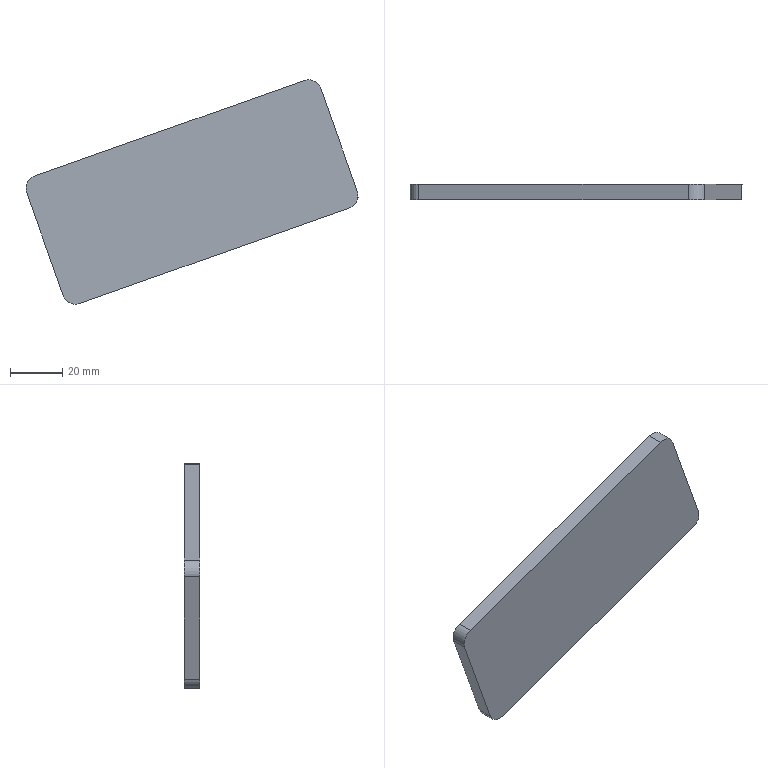Part | STEP file | WEAR-PLATE1_id194_x_t | 1 solid | 10 faces | box 127.71 x 6 x 86.31 mm | volume 37311 mm3 | plane 6 | cylinder 4 | commonest cylinder face diameters 10 x4
STEP:
#1=CARTESIAN_POINT('',(-15.423,-66.,-192.471));
#2=VERTEX_POINT('',#1);
#3=CARTESIAN_POINT('',(-12.379,-66.,-186.088));
#4=VERTEX_POINT('',#3);
#5=CARTESIAN_POINT('',(-10.71,-66.,-190.802));
#6=DIRECTION('',(0.,1.,0.));
#7=DIRECTION('',(0.,0.,1.));
#8=AXIS2_PLACEMENT_3D('',#5,#6,#7);
#9=CIRCLE('',#8,5.);
#10=EDGE_CURVE('',#2,#4,#9,.T.);
#11=ORIENTED_EDGE('',*,*,#10,.F.);
#12=CARTESIAN_POINT('',(-1.403,-66.,-232.062));
#13=VERTEX_POINT('',#12);
#14=CARTESIAN_POINT('',(-1.403,-66.,-232.062));
#15=DIRECTION('',(-0.3338,0.,0.9426));
#16=VECTOR('',#15,1.);
#17=LINE('',#14,#16);
#18=EDGE_CURVE('',#13,#2,#17,.T.);
#19=ORIENTED_EDGE('',*,*,#18,.F.);
#20=CARTESIAN_POINT('',(4.979,-66.,-235.106));
#21=VERTEX_POINT('',#20);
#22=CARTESIAN_POINT('',(3.31,-66.,-230.393));
#23=DIRECTION('',(0.,1.,0.));
#24=DIRECTION('',(0.,0.,1.));
#25=AXIS2_PLACEMENT_3D('',#22,#23,#24);
#26=CIRCLE('',#25,5.);
#27=EDGE_CURVE('',#21,#13,#26,.T.);
#28=ORIENTED_EDGE('',*,*,#27,.F.);
#29=CARTESIAN_POINT('',(108.669,-66.,-198.387));
#30=VERTEX_POINT('',#29);
#31=CARTESIAN_POINT('',(108.669,-66.,-198.387));
#32=DIRECTION('',(-0.9426,0.,-0.3338));
#33=VECTOR('',#32,1.);
#34=LINE('',#31,#33);
#35=EDGE_CURVE('',#30,#21,#34,.T.);
#36=ORIENTED_EDGE('',*,*,#35,.F.);
#37=CARTESIAN_POINT('',(111.714,-66.,-192.005));
#38=VERTEX_POINT('',#37);
#39=CARTESIAN_POINT('',(107.,-66.,-193.674));
#40=DIRECTION('',(0.,1.,0.));
#41=DIRECTION('',(0.,0.,1.));
#42=AXIS2_PLACEMENT_3D('',#39,#40,#41);
#43=CIRCLE('',#42,5.);
#44=EDGE_CURVE('',#38,#30,#43,.T.);
#45=ORIENTED_EDGE('',*,*,#44,.F.);
#46=CARTESIAN_POINT('',(97.694,-66.,-152.414));
#47=VERTEX_POINT('',#46);
#48=CARTESIAN_POINT('',(97.694,-66.,-152.414));
#49=DIRECTION('',(0.3338,0.,-0.9426));
#50=VECTOR('',#49,1.);
#51=LINE('',#48,#50);
#52=EDGE_CURVE('',#47,#38,#51,.T.);
#53=ORIENTED_EDGE('',*,*,#52,.F.);
#54=CARTESIAN_POINT('',(91.311,-66.,-149.37));
#55=VERTEX_POINT('',#54);
#56=CARTESIAN_POINT('',(92.981,-66.,-154.083));
#57=DIRECTION('',(0.,1.,0.));
#58=DIRECTION('',(0.,0.,1.));
#59=AXIS2_PLACEMENT_3D('',#56,#57,#58);
#60=CIRCLE('',#59,5.);
#61=EDGE_CURVE('',#55,#47,#60,.T.);
#62=ORIENTED_EDGE('',*,*,#61,.F.);
#63=CARTESIAN_POINT('',(-12.379,-66.,-186.088));
#64=DIRECTION('',(0.9426,0.,0.3338));
#65=VECTOR('',#64,1.);
#66=LINE('',#63,#65);
#67=EDGE_CURVE('',#4,#55,#66,.T.);
#68=ORIENTED_EDGE('',*,*,#67,.F.);
#69=EDGE_LOOP('',(#11,#19,#28,#36,#45,#53,#62,#68));
#70=FACE_OUTER_BOUND('',#69,.T.);
#71=CARTESIAN_POINT('',(-200.,-66.,-275.));
#72=DIRECTION('',(0.,1.,0.));
#73=DIRECTION('',(0.,0.,1.));
#74=AXIS2_PLACEMENT_3D('',#71,#72,#73);
#75=PLANE('',#74);
#76=ADVANCED_FACE('',(#70),#75,.F.);
#77=CARTESIAN_POINT('',(91.311,-60.,-149.37));
#78=VERTEX_POINT('',#77);
#79=CARTESIAN_POINT('',(91.311,-66.,-149.37));
#80=DIRECTION('',(0.,1.,0.));
#81=VECTOR('',#80,1.);
#82=LINE('',#79,#81);
#83=EDGE_CURVE('',#55,#78,#82,.T.);
#84=ORIENTED_EDGE('',*,*,#83,.F.);
#85=ORIENTED_EDGE('',*,*,#61,.T.);
#86=CARTESIAN_POINT('',(97.694,-60.,-152.414));
#87=VERTEX_POINT('',#86);
#88=CARTESIAN_POINT('',(97.694,-66.,-152.414));
#89=DIRECTION('',(0.,-1.,0.));
#90=VECTOR('',#89,1.);
#91=LINE('',#88,#90);
#92=EDGE_CURVE('',#87,#47,#91,.T.);
#93=ORIENTED_EDGE('',*,*,#92,.F.);
#94=CARTESIAN_POINT('',(92.981,-60.,-154.083));
#95=DIRECTION('',(0.,-1.,0.));
#96=DIRECTION('',(0.,0.,1.));
#97=AXIS2_PLACEMENT_3D('',#94,#95,#96);
#98=CIRCLE('',#97,5.);
#99=EDGE_CURVE('',#87,#78,#98,.T.);
#100=ORIENTED_EDGE('',*,*,#99,.T.);
#101=EDGE_LOOP('',(#84,#85,#93,#100));
#102=FACE_OUTER_BOUND('',#101,.T.);
#103=CARTESIAN_POINT('',(92.981,-66.,-154.083));
#104=DIRECTION('',(0.,1.,0.));
#105=DIRECTION('',(0.,0.,1.));
#106=AXIS2_PLACEMENT_3D('',#103,#104,#105);
#107=CYLINDRICAL_SURFACE('',#106,5.);
#108=ADVANCED_FACE('',(#102),#107,.T.);
#109=CARTESIAN_POINT('',(-12.379,-60.,-186.088));
#110=VERTEX_POINT('',#109);
#111=CARTESIAN_POINT('',(-12.379,-66.,-186.088));
#112=DIRECTION('',(0.,1.,0.));
#113=VECTOR('',#112,1.);
#114=LINE('',#111,#113);
#115=EDGE_CURVE('',#4,#110,#114,.T.);
#116=ORIENTED_EDGE('',*,*,#115,.F.);
#117=ORIENTED_EDGE('',*,*,#67,.T.);
#118=ORIENTED_EDGE('',*,*,#83,.T.);
#119=CARTESIAN_POINT('',(91.311,-60.,-149.37));
#120=DIRECTION('',(-0.9426,0.,-0.3338));
#121=VECTOR('',#120,1.);
#122=LINE('',#119,#121);
#123=EDGE_CURVE('',#78,#110,#122,.T.);
#124=ORIENTED_EDGE('',*,*,#123,.T.);
#125=EDGE_LOOP('',(#116,#117,#118,#124));
#126=FACE_OUTER_BOUND('',#125,.T.);
#127=CARTESIAN_POINT('',(-12.379,-66.,-186.088));
#128=DIRECTION('',(-0.3338,0.,0.9426));
#129=DIRECTION('',(0.9426,0.,0.3338));
#130=AXIS2_PLACEMENT_3D('',#127,#128,#129);
#131=PLANE('',#130);
#132=ADVANCED_FACE('',(#126),#131,.T.);
#133=CARTESIAN_POINT('',(-15.423,-60.,-192.471));
#134=VERTEX_POINT('',#133);
#135=CARTESIAN_POINT('',(-15.423,-66.,-192.471));
#136=DIRECTION('',(0.,1.,0.));
#137=VECTOR('',#136,1.);
#138=LINE('',#135,#137);
#139=EDGE_CURVE('',#2,#134,#138,.T.);
#140=ORIENTED_EDGE('',*,*,#139,.F.);
#141=ORIENTED_EDGE('',*,*,#10,.T.);
#142=ORIENTED_EDGE('',*,*,#115,.T.);
#143=CARTESIAN_POINT('',(-10.71,-60.,-190.802));
#144=DIRECTION('',(0.,-1.,0.));
#145=DIRECTION('',(0.,0.,1.));
#146=AXIS2_PLACEMENT_3D('',#143,#144,#145);
#147=CIRCLE('',#146,5.);
#148=EDGE_CURVE('',#110,#134,#147,.T.);
#149=ORIENTED_EDGE('',*,*,#148,.T.);
#150=EDGE_LOOP('',(#140,#141,#142,#149));
#151=FACE_OUTER_BOUND('',#150,.T.);
#152=CARTESIAN_POINT('',(-10.71,-66.,-190.802));
#153=DIRECTION('',(0.,1.,0.));
#154=DIRECTION('',(0.,0.,1.));
#155=AXIS2_PLACEMENT_3D('',#152,#153,#154);
#156=CYLINDRICAL_SURFACE('',#155,5.);
#157=ADVANCED_FACE('',(#151),#156,.T.);
#158=CARTESIAN_POINT('',(-1.403,-60.,-232.062));
#159=VERTEX_POINT('',#158);
#160=CARTESIAN_POINT('',(-1.403,-66.,-232.062));
#161=DIRECTION('',(0.,1.,0.));
#162=VECTOR('',#161,1.);
#163=LINE('',#160,#162);
#164=EDGE_CURVE('',#13,#159,#163,.T.);
#165=ORIENTED_EDGE('',*,*,#164,.F.);
#166=ORIENTED_EDGE('',*,*,#18,.T.);
#167=ORIENTED_EDGE('',*,*,#139,.T.);
#168=CARTESIAN_POINT('',(-15.423,-60.,-192.471));
#169=DIRECTION('',(0.3338,0.,-0.9426));
#170=VECTOR('',#169,1.);
#171=LINE('',#168,#170);
#172=EDGE_CURVE('',#134,#159,#171,.T.);
#173=ORIENTED_EDGE('',*,*,#172,.T.);
#174=EDGE_LOOP('',(#165,#166,#167,#173));
#175=FACE_OUTER_BOUND('',#174,.T.);
#176=CARTESIAN_POINT('',(-1.403,-66.,-232.062));
#177=DIRECTION('',(-0.9426,0.,-0.3338));
#178=DIRECTION('',(-0.3338,0.,0.9426));
#179=AXIS2_PLACEMENT_3D('',#176,#177,#178);
#180=PLANE('',#179);
#181=ADVANCED_FACE('',(#175),#180,.T.);
#182=CARTESIAN_POINT('',(4.979,-60.,-235.106));
#183=VERTEX_POINT('',#182);
#184=CARTESIAN_POINT('',(4.979,-66.,-235.106));
#185=DIRECTION('',(0.,1.,0.));
#186=VECTOR('',#185,1.);
#187=LINE('',#184,#186);
#188=EDGE_CURVE('',#21,#183,#187,.T.);
#189=ORIENTED_EDGE('',*,*,#188,.F.);
#190=ORIENTED_EDGE('',*,*,#27,.T.);
#191=ORIENTED_EDGE('',*,*,#164,.T.);
#192=CARTESIAN_POINT('',(3.31,-60.,-230.393));
#193=DIRECTION('',(0.,-1.,0.));
#194=DIRECTION('',(0.,0.,1.));
#195=AXIS2_PLACEMENT_3D('',#192,#193,#194);
#196=CIRCLE('',#195,5.);
#197=EDGE_CURVE('',#159,#183,#196,.T.);
#198=ORIENTED_EDGE('',*,*,#197,.T.);
#199=EDGE_LOOP('',(#189,#190,#191,#198));
#200=FACE_OUTER_BOUND('',#199,.T.);
#201=CARTESIAN_POINT('',(3.31,-66.,-230.393));
#202=DIRECTION('',(0.,1.,0.));
#203=DIRECTION('',(0.,0.,1.));
#204=AXIS2_PLACEMENT_3D('',#201,#202,#203);
#205=CYLINDRICAL_SURFACE('',#204,5.);
#206=ADVANCED_FACE('',(#200),#205,.T.);
#207=CARTESIAN_POINT('',(108.669,-60.,-198.387));
#208=VERTEX_POINT('',#207);
#209=CARTESIAN_POINT('',(108.669,-66.,-198.387));
#210=DIRECTION('',(0.,1.,0.));
#211=VECTOR('',#210,1.);
#212=LINE('',#209,#211);
#213=EDGE_CURVE('',#30,#208,#212,.T.);
#214=ORIENTED_EDGE('',*,*,#213,.F.);
#215=ORIENTED_EDGE('',*,*,#35,.T.);
#216=ORIENTED_EDGE('',*,*,#188,.T.);
#217=CARTESIAN_POINT('',(4.979,-60.,-235.106));
#218=DIRECTION('',(0.9426,0.,0.3338));
#219=VECTOR('',#218,1.);
#220=LINE('',#217,#219);
#221=EDGE_CURVE('',#183,#208,#220,.T.);
#222=ORIENTED_EDGE('',*,*,#221,.T.);
#223=EDGE_LOOP('',(#214,#215,#216,#222));
#224=FACE_OUTER_BOUND('',#223,.T.);
#225=CARTESIAN_POINT('',(108.669,-66.,-198.387));
#226=DIRECTION('',(0.3338,0.,-0.9426));
#227=DIRECTION('',(-0.9426,0.,-0.3338));
#228=AXIS2_PLACEMENT_3D('',#225,#226,#227);
#229=PLANE('',#228);
#230=ADVANCED_FACE('',(#224),#229,.T.);
#231=CARTESIAN_POINT('',(111.714,-60.,-192.005));
#232=VERTEX_POINT('',#231);
#233=CARTESIAN_POINT('',(111.714,-66.,-192.005));
#234=DIRECTION('',(0.,1.,0.));
#235=VECTOR('',#234,1.);
#236=LINE('',#233,#235);
#237=EDGE_CURVE('',#38,#232,#236,.T.);
#238=ORIENTED_EDGE('',*,*,#237,.F.);
#239=ORIENTED_EDGE('',*,*,#44,.T.);
#240=ORIENTED_EDGE('',*,*,#213,.T.);
#241=CARTESIAN_POINT('',(107.,-60.,-193.674));
#242=DIRECTION('',(0.,-1.,0.));
#243=DIRECTION('',(0.,0.,1.));
#244=AXIS2_PLACEMENT_3D('',#241,#242,#243);
#245=CIRCLE('',#244,5.);
#246=EDGE_CURVE('',#208,#232,#245,.T.);
#247=ORIENTED_EDGE('',*,*,#246,.T.);
#248=EDGE_LOOP('',(#238,#239,#240,#247));
#249=FACE_OUTER_BOUND('',#248,.T.);
#250=CARTESIAN_POINT('',(107.,-66.,-193.674));
#251=DIRECTION('',(0.,1.,0.));
#252=DIRECTION('',(0.,0.,1.));
#253=AXIS2_PLACEMENT_3D('',#250,#251,#252);
#254=CYLINDRICAL_SURFACE('',#253,5.);
#255=ADVANCED_FACE('',(#249),#254,.T.);
#256=ORIENTED_EDGE('',*,*,#92,.T.);
#257=ORIENTED_EDGE('',*,*,#52,.T.);
#258=ORIENTED_EDGE('',*,*,#237,.T.);
#259=CARTESIAN_POINT('',(111.714,-60.,-192.005));
#260=DIRECTION('',(-0.3338,0.,0.9426));
#261=VECTOR('',#260,1.);
#262=LINE('',#259,#261);
#263=EDGE_CURVE('',#232,#87,#262,.T.);
#264=ORIENTED_EDGE('',*,*,#263,.T.);
#265=EDGE_LOOP('',(#256,#257,#258,#264));
#266=FACE_OUTER_BOUND('',#265,.T.);
#267=CARTESIAN_POINT('',(97.694,-66.,-152.414));
#268=DIRECTION('',(0.9426,0.,0.3338));
#269=DIRECTION('',(0.3338,0.,-0.9426));
#270=AXIS2_PLACEMENT_3D('',#267,#268,#269);
#271=PLANE('',#270);
#272=ADVANCED_FACE('',(#266),#271,.T.);
#273=ORIENTED_EDGE('',*,*,#246,.F.);
#274=ORIENTED_EDGE('',*,*,#221,.F.);
#275=ORIENTED_EDGE('',*,*,#197,.F.);
#276=ORIENTED_EDGE('',*,*,#172,.F.);
#277=ORIENTED_EDGE('',*,*,#148,.F.);
#278=ORIENTED_EDGE('',*,*,#123,.F.);
#279=ORIENTED_EDGE('',*,*,#99,.F.);
#280=ORIENTED_EDGE('',*,*,#263,.F.);
#281=EDGE_LOOP('',(#273,#274,#275,#276,#277,#278,#279,#280));
#282=FACE_OUTER_BOUND('',#281,.T.);
#283=CARTESIAN_POINT('',(-80.,-60.,-43.));
#284=DIRECTION('',(0.,-1.,0.));
#285=DIRECTION('',(0.,0.,-1.));
#286=AXIS2_PLACEMENT_3D('',#283,#284,#285);
#287=PLANE('',#286);
#288=ADVANCED_FACE('',(#282),#287,.F.);
#289=CLOSED_SHELL('',(#76,#108,#132,#157,#181,#206,#230,#255,#272,#288));
#290=MANIFOLD_SOLID_BREP('',#289);
#291=(LENGTH_UNIT()NAMED_UNIT(*)SI_UNIT(.MILLI.,.METRE.));
#292=UNCERTAINTY_MEASURE_WITH_UNIT(LENGTH_MEASURE(0.00002),#291,'','');
#293=(NAMED_UNIT(*)PLANE_ANGLE_UNIT()SI_UNIT($,.RADIAN.));
#294=PLANE_ANGLE_MEASURE_WITH_UNIT(PLANE_ANGLE_MEASURE(0.01745),#293);
#295=DIMENSIONAL_EXPONENTS(0.,0.,0.,0.,0.,0.,0.);
#296=(CONVERSION_BASED_UNIT('DEGREE',#294)NAMED_UNIT(#295)PLANE_ANGLE_UNIT());
#297=(NAMED_UNIT(*)SI_UNIT($,.STERADIAN.)SOLID_ANGLE_UNIT());
#298=(GEOMETRIC_REPRESENTATION_CONTEXT(3)GLOBAL_UNCERTAINTY_ASSIGNED_CONTEXT((#292))GLOBAL_UNIT_ASSIGNED_CONTEXT((#291,#296,#297))REPRESENTATION_CONTEXT('',''));
#299=ADVANCED_BREP_SHAPE_REPRESENTATION('',(#290),#298);